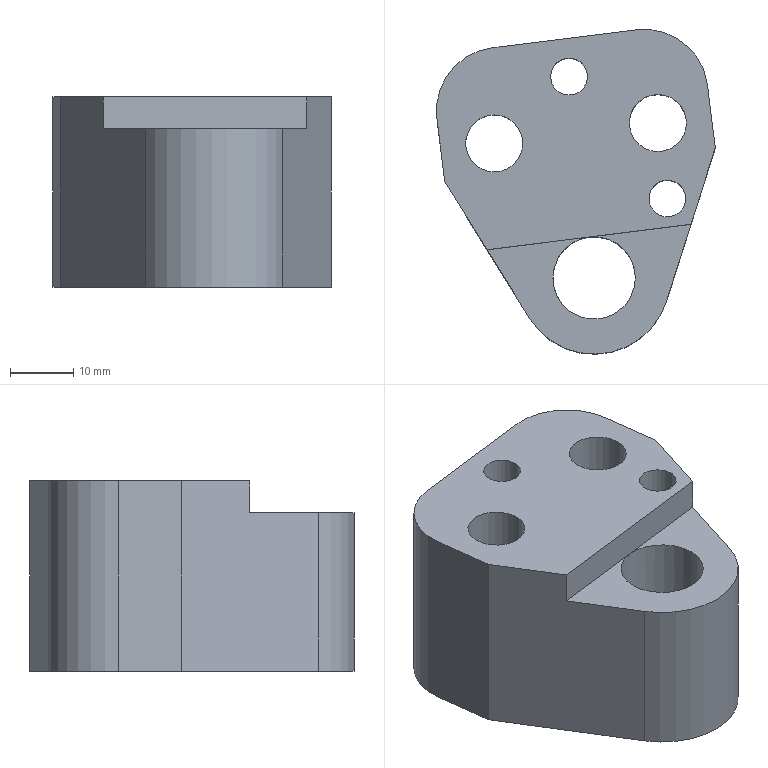Part | NX | features CP-FP 13 2 | 1 solid | 21 faces | box 43.983 x 51.207 x 30 mm | volume 37532 mm3 | plane 11 | cylinder 10 | commonest cylinder face diameters 5.8 x2 9 x2 14 x2 20 x2 13 x1 24 x1
STEP:
#1=CARTESIAN_POINT('',(623.685,-6.896,49.));
#2=VERTEX_POINT('',#1);
#3=CARTESIAN_POINT('',(624.921,-16.819,49.));
#4=VERTEX_POINT('',#3);
#5=CARTESIAN_POINT('',(622.449,3.027,49.));
#6=DIRECTION('',(0.1236,-0.9923,0.));
#7=VECTOR('',#6,1000.);
#8=LINE('',#5,#7);
#9=EDGE_CURVE('',#2,#4,#8,.T.);
#10=ORIENTED_EDGE('',*,*,#9,.F.);
#11=CARTESIAN_POINT('',(623.685,-6.896,79.));
#12=VERTEX_POINT('',#11);
#13=CARTESIAN_POINT('',(623.685,-6.896,49.));
#14=DIRECTION('',(0.,0.,1.));
#15=VECTOR('',#14,1000.);
#16=LINE('',#13,#15);
#17=EDGE_CURVE('',#2,#12,#16,.T.);
#18=ORIENTED_EDGE('',*,*,#17,.T.);
#19=CARTESIAN_POINT('',(624.921,-16.819,79.));
#20=VERTEX_POINT('',#19);
#21=CARTESIAN_POINT('',(622.449,3.027,79.));
#22=DIRECTION('',(0.1236,-0.9923,0.));
#23=VECTOR('',#22,1000.);
#24=LINE('',#21,#23);
#25=EDGE_CURVE('',#12,#20,#24,.T.);
#26=ORIENTED_EDGE('',*,*,#25,.T.);
#27=CARTESIAN_POINT('',(624.921,-16.819,49.));
#28=DIRECTION('',(0.,0.,1.));
#29=VECTOR('',#28,1000.);
#30=LINE('',#27,#29);
#31=EDGE_CURVE('',#4,#20,#30,.T.);
#32=ORIENTED_EDGE('',*,*,#31,.F.);
#33=EDGE_LOOP('',(#10,#18,#26,#32));
#34=FACE_BOUND('',#33,.T.);
#35=CARTESIAN_POINT('',(622.449,3.027,49.));
#36=DIRECTION('',(-0.9923,-0.1236,0.));
#37=DIRECTION('',(0.1236,-0.9923,0.));
#38=AXIS2_PLACEMENT_3D('',#35,#36,#37);
#39=PLANE('',#38);
#40=ADVANCED_FACE('',(#34),#39,.F.);
#41=CARTESIAN_POINT('',(621.088,-28.886,79.));
#42=VERTEX_POINT('',#41);
#43=CARTESIAN_POINT('',(621.088,-28.886,74.));
#44=VERTEX_POINT('',#43);
#45=CARTESIAN_POINT('',(621.088,-28.886,49.));
#46=DIRECTION('',(0.,0.,-1.));
#47=VECTOR('',#46,1000.);
#48=LINE('',#45,#47);
#49=EDGE_CURVE('',#42,#44,#48,.T.);
#50=ORIENTED_EDGE('',*,*,#49,.T.);
#51=CARTESIAN_POINT('',(617.248,-40.972,74.));
#52=VERTEX_POINT('',#51);
#53=CARTESIAN_POINT('',(624.921,-16.819,74.));
#54=DIRECTION('',(-0.3028,-0.9531,0.));
#55=VECTOR('',#54,1000.);
#56=LINE('',#53,#55);
#57=EDGE_CURVE('',#44,#52,#56,.T.);
#58=ORIENTED_EDGE('',*,*,#57,.T.);
#59=CARTESIAN_POINT('',(617.248,-40.972,49.));
#60=VERTEX_POINT('',#59);
#61=CARTESIAN_POINT('',(617.248,-40.972,49.));
#62=DIRECTION('',(0.,0.,1.));
#63=VECTOR('',#62,1000.);
#64=LINE('',#61,#63);
#65=EDGE_CURVE('',#60,#52,#64,.T.);
#66=ORIENTED_EDGE('',*,*,#65,.F.);
#67=CARTESIAN_POINT('',(624.921,-16.819,49.));
#68=DIRECTION('',(-0.3028,-0.9531,0.));
#69=VECTOR('',#68,1000.);
#70=LINE('',#67,#69);
#71=EDGE_CURVE('',#4,#60,#70,.T.);
#72=ORIENTED_EDGE('',*,*,#71,.F.);
#73=ORIENTED_EDGE('',*,*,#31,.T.);
#74=CARTESIAN_POINT('',(624.921,-16.819,79.));
#75=DIRECTION('',(-0.3028,-0.9531,0.));
#76=VECTOR('',#75,1000.);
#77=LINE('',#74,#76);
#78=EDGE_CURVE('',#20,#42,#77,.T.);
#79=ORIENTED_EDGE('',*,*,#78,.T.);
#80=EDGE_LOOP('',(#50,#58,#66,#72,#73,#79));
#81=FACE_BOUND('',#80,.T.);
#82=CARTESIAN_POINT('',(624.921,-16.819,49.));
#83=DIRECTION('',(-0.9531,0.3028,0.));
#84=DIRECTION('',(-0.3028,-0.9531,0.));
#85=AXIS2_PLACEMENT_3D('',#82,#83,#84);
#86=PLANE('',#85);
#87=ADVANCED_FACE('',(#81),#86,.F.);
#88=CARTESIAN_POINT('',(595.616,-43.668,74.));
#89=VERTEX_POINT('',#88);
#90=CARTESIAN_POINT('',(605.812,-37.339,74.));
#91=DIRECTION('',(0.,0.,-1.));
#92=DIRECTION('',(0.,1.,0.));
#93=AXIS2_PLACEMENT_3D('',#90,#91,#92);
#94=CIRCLE('',#93,12.);
#95=EDGE_CURVE('',#89,#52,#94,.F.);
#96=ORIENTED_EDGE('',*,*,#95,.F.);
#97=CARTESIAN_POINT('',(595.616,-43.668,49.));
#98=VERTEX_POINT('',#97);
#99=CARTESIAN_POINT('',(595.616,-43.668,49.));
#100=DIRECTION('',(0.,0.,1.));
#101=VECTOR('',#100,1000.);
#102=LINE('',#99,#101);
#103=EDGE_CURVE('',#98,#89,#102,.T.);
#104=ORIENTED_EDGE('',*,*,#103,.F.);
#105=CARTESIAN_POINT('',(605.812,-37.339,49.));
#106=DIRECTION('',(0.,0.,1.));
#107=DIRECTION('',(0.,-1.,0.));
#108=AXIS2_PLACEMENT_3D('',#105,#106,#107);
#109=CIRCLE('',#108,12.);
#110=EDGE_CURVE('',#98,#60,#109,.T.);
#111=ORIENTED_EDGE('',*,*,#110,.T.);
#112=ORIENTED_EDGE('',*,*,#65,.T.);
#113=EDGE_LOOP('',(#96,#104,#111,#112));
#114=FACE_BOUND('',#113,.T.);
#115=CARTESIAN_POINT('',(605.812,-37.339,49.));
#116=DIRECTION('',(0.,0.,1.));
#117=DIRECTION('',(0.,-1.,0.));
#118=AXIS2_PLACEMENT_3D('',#115,#116,#117);
#119=CYLINDRICAL_SURFACE('',#118,12.);
#120=ADVANCED_FACE('',(#114),#119,.T.);
#121=CARTESIAN_POINT('',(588.928,-32.893,74.));
#122=VERTEX_POINT('',#121);
#123=CARTESIAN_POINT('',(582.251,-22.136,74.));
#124=DIRECTION('',(0.5274,-0.8496,0.));
#125=VECTOR('',#124,1000.);
#126=LINE('',#123,#125);
#127=EDGE_CURVE('',#122,#89,#126,.T.);
#128=ORIENTED_EDGE('',*,*,#127,.F.);
#129=CARTESIAN_POINT('',(588.928,-32.893,79.));
#130=VERTEX_POINT('',#129);
#131=CARTESIAN_POINT('',(588.928,-32.893,49.));
#132=DIRECTION('',(0.,0.,-1.));
#133=VECTOR('',#132,1000.);
#134=LINE('',#131,#133);
#135=EDGE_CURVE('',#130,#122,#134,.T.);
#136=ORIENTED_EDGE('',*,*,#135,.F.);
#137=CARTESIAN_POINT('',(582.251,-22.136,79.));
#138=VERTEX_POINT('',#137);
#139=CARTESIAN_POINT('',(582.251,-22.136,79.));
#140=DIRECTION('',(0.5274,-0.8496,0.));
#141=VECTOR('',#140,1000.);
#142=LINE('',#139,#141);
#143=EDGE_CURVE('',#138,#130,#142,.T.);
#144=ORIENTED_EDGE('',*,*,#143,.F.);
#145=CARTESIAN_POINT('',(582.251,-22.136,49.));
#146=VERTEX_POINT('',#145);
#147=CARTESIAN_POINT('',(582.251,-22.136,49.));
#148=DIRECTION('',(0.,0.,1.));
#149=VECTOR('',#148,1000.);
#150=LINE('',#147,#149);
#151=EDGE_CURVE('',#146,#138,#150,.T.);
#152=ORIENTED_EDGE('',*,*,#151,.F.);
#153=CARTESIAN_POINT('',(582.251,-22.136,49.));
#154=DIRECTION('',(0.5274,-0.8496,0.));
#155=VECTOR('',#154,1000.);
#156=LINE('',#153,#155);
#157=EDGE_CURVE('',#146,#98,#156,.T.);
#158=ORIENTED_EDGE('',*,*,#157,.T.);
#159=ORIENTED_EDGE('',*,*,#103,.T.);
#160=EDGE_LOOP('',(#128,#136,#144,#152,#158,#159));
#161=FACE_BOUND('',#160,.T.);
#162=CARTESIAN_POINT('',(582.251,-22.136,49.));
#163=DIRECTION('',(-0.8496,-0.5274,0.));
#164=DIRECTION('',(0.5274,-0.8496,0.));
#165=AXIS2_PLACEMENT_3D('',#162,#163,#164);
#166=PLANE('',#165);
#167=ADVANCED_FACE('',(#161),#166,.T.);
#168=CARTESIAN_POINT('',(581.015,-12.212,79.));
#169=VERTEX_POINT('',#168);
#170=CARTESIAN_POINT('',(579.778,-2.289,79.));
#171=DIRECTION('',(0.1236,-0.9923,0.));
#172=VECTOR('',#171,1000.);
#173=LINE('',#170,#172);
#174=EDGE_CURVE('',#169,#138,#173,.T.);
#175=ORIENTED_EDGE('',*,*,#174,.F.);
#176=CARTESIAN_POINT('',(581.015,-12.212,49.));
#177=VERTEX_POINT('',#176);
#178=CARTESIAN_POINT('',(581.015,-12.212,49.));
#179=DIRECTION('',(0.,0.,1.));
#180=VECTOR('',#179,1000.);
#181=LINE('',#178,#180);
#182=EDGE_CURVE('',#169,#177,#181,.F.);
#183=ORIENTED_EDGE('',*,*,#182,.T.);
#184=CARTESIAN_POINT('',(579.778,-2.289,49.));
#185=DIRECTION('',(0.1236,-0.9923,0.));
#186=VECTOR('',#185,1000.);
#187=LINE('',#184,#186);
#188=EDGE_CURVE('',#177,#146,#187,.T.);
#189=ORIENTED_EDGE('',*,*,#188,.T.);
#190=ORIENTED_EDGE('',*,*,#151,.T.);
#191=EDGE_LOOP('',(#175,#183,#189,#190));
#192=FACE_BOUND('',#191,.T.);
#193=CARTESIAN_POINT('',(579.778,-2.289,49.));
#194=DIRECTION('',(-0.9923,-0.1236,0.));
#195=DIRECTION('',(0.1236,-0.9923,0.));
#196=AXIS2_PLACEMENT_3D('',#193,#194,#195);
#197=PLANE('',#196);
#198=ADVANCED_FACE('',(#192),#197,.T.);
#199=CARTESIAN_POINT('',(589.702,-1.053,79.));
#200=VERTEX_POINT('',#199);
#201=CARTESIAN_POINT('',(612.525,1.791,79.));
#202=VERTEX_POINT('',#201);
#203=CARTESIAN_POINT('',(579.778,-2.289,79.));
#204=DIRECTION('',(0.9923,0.1236,0.));
#205=VECTOR('',#204,1000.);
#206=LINE('',#203,#205);
#207=EDGE_CURVE('',#200,#202,#206,.T.);
#208=ORIENTED_EDGE('',*,*,#207,.T.);
#209=CARTESIAN_POINT('',(612.525,1.791,49.));
#210=VERTEX_POINT('',#209);
#211=CARTESIAN_POINT('',(612.525,1.791,49.));
#212=DIRECTION('',(0.,0.,1.));
#213=VECTOR('',#212,1000.);
#214=LINE('',#211,#213);
#215=EDGE_CURVE('',#202,#210,#214,.F.);
#216=ORIENTED_EDGE('',*,*,#215,.T.);
#217=CARTESIAN_POINT('',(589.702,-1.053,49.));
#218=VERTEX_POINT('',#217);
#219=CARTESIAN_POINT('',(579.778,-2.289,49.));
#220=DIRECTION('',(0.9923,0.1236,0.));
#221=VECTOR('',#220,1000.);
#222=LINE('',#219,#221);
#223=EDGE_CURVE('',#218,#210,#222,.T.);
#224=ORIENTED_EDGE('',*,*,#223,.F.);
#225=CARTESIAN_POINT('',(589.702,-1.053,79.));
#226=DIRECTION('',(0.,0.,1.));
#227=VECTOR('',#226,1000.);
#228=LINE('',#225,#227);
#229=EDGE_CURVE('',#218,#200,#228,.T.);
#230=ORIENTED_EDGE('',*,*,#229,.T.);
#231=EDGE_LOOP('',(#208,#216,#224,#230));
#232=FACE_BOUND('',#231,.T.);
#233=CARTESIAN_POINT('',(579.778,-2.289,49.));
#234=DIRECTION('',(0.1236,-0.9923,0.));
#235=DIRECTION('',(0.9923,0.1236,0.));
#236=AXIS2_PLACEMENT_3D('',#233,#234,#235);
#237=PLANE('',#236);
#238=ADVANCED_FACE('',(#232),#237,.F.);
#239=CARTESIAN_POINT('',(615.868,-19.909,49.));
#240=VERTEX_POINT('',#239);
#241=CARTESIAN_POINT('',(615.868,-12.909,49.));
#242=DIRECTION('',(0.,0.,1.));
#243=DIRECTION('',(0.,-1.,0.));
#244=AXIS2_PLACEMENT_3D('',#241,#242,#243);
#245=CIRCLE('',#244,7.);
#246=EDGE_CURVE('',#240,#240,#245,.T.);
#247=ORIENTED_EDGE('',*,*,#246,.T.);
#248=EDGE_LOOP('',(#247));
#249=FACE_BOUND('',#248,.T.);
#250=CARTESIAN_POINT('',(590.068,-23.123,49.));
#251=VERTEX_POINT('',#250);
#252=CARTESIAN_POINT('',(590.068,-16.123,49.));
#253=DIRECTION('',(0.,0.,1.));
#254=DIRECTION('',(0.,-1.,0.));
#255=AXIS2_PLACEMENT_3D('',#252,#253,#254);
#256=CIRCLE('',#255,7.);
#257=EDGE_CURVE('',#251,#251,#256,.T.);
#258=ORIENTED_EDGE('',*,*,#257,.T.);
#259=EDGE_LOOP('',(#258));
#260=FACE_BOUND('',#259,.T.);
#261=CARTESIAN_POINT('',(617.352,-27.716,49.));
#262=VERTEX_POINT('',#261);
#263=CARTESIAN_POINT('',(617.352,-24.816,49.));
#264=DIRECTION('',(0.,0.,1.));
#265=DIRECTION('',(0.,-1.,0.));
#266=AXIS2_PLACEMENT_3D('',#263,#264,#265);
#267=CIRCLE('',#266,2.9);
#268=EDGE_CURVE('',#262,#262,#267,.T.);
#269=ORIENTED_EDGE('',*,*,#268,.T.);
#270=EDGE_LOOP('',(#269));
#271=FACE_BOUND('',#270,.T.);
#272=CARTESIAN_POINT('',(601.855,-8.485,49.));
#273=VERTEX_POINT('',#272);
#274=CARTESIAN_POINT('',(601.855,-5.585,49.));
#275=DIRECTION('',(0.,0.,1.));
#276=DIRECTION('',(0.,-1.,0.));
#277=AXIS2_PLACEMENT_3D('',#274,#275,#276);
#278=CIRCLE('',#277,2.9);
#279=EDGE_CURVE('',#273,#273,#278,.T.);
#280=ORIENTED_EDGE('',*,*,#279,.T.);
#281=EDGE_LOOP('',(#280));
#282=FACE_BOUND('',#281,.T.);
#283=CARTESIAN_POINT('',(605.812,-43.839,49.));
#284=VERTEX_POINT('',#283);
#285=CARTESIAN_POINT('',(605.812,-37.339,49.));
#286=DIRECTION('',(0.,0.,1.));
#287=DIRECTION('',(0.,-1.,0.));
#288=AXIS2_PLACEMENT_3D('',#285,#286,#287);
#289=CIRCLE('',#288,6.5);
#290=EDGE_CURVE('',#284,#284,#289,.T.);
#291=ORIENTED_EDGE('',*,*,#290,.T.);
#292=EDGE_LOOP('',(#291));
#293=FACE_BOUND('',#292,.T.);
#294=ORIENTED_EDGE('',*,*,#223,.T.);
#295=CARTESIAN_POINT('',(613.762,-8.132,49.));
#296=DIRECTION('',(0.,0.,1.));
#297=DIRECTION('',(0.,-1.,0.));
#298=AXIS2_PLACEMENT_3D('',#295,#296,#297);
#299=CIRCLE('',#298,10.);
#300=EDGE_CURVE('',#210,#2,#299,.F.);
#301=ORIENTED_EDGE('',*,*,#300,.T.);
#302=ORIENTED_EDGE('',*,*,#9,.T.);
#303=ORIENTED_EDGE('',*,*,#71,.T.);
#304=ORIENTED_EDGE('',*,*,#110,.F.);
#305=ORIENTED_EDGE('',*,*,#157,.F.);
#306=ORIENTED_EDGE('',*,*,#188,.F.);
#307=CARTESIAN_POINT('',(590.938,-10.976,49.));
#308=DIRECTION('',(0.,0.,1.));
#309=DIRECTION('',(0.,-1.,0.));
#310=AXIS2_PLACEMENT_3D('',#307,#308,#309);
#311=CIRCLE('',#310,10.);
#312=EDGE_CURVE('',#177,#218,#311,.F.);
#313=ORIENTED_EDGE('',*,*,#312,.T.);
#314=EDGE_LOOP('',(#294,#301,#302,#303,#304,#305,#306,#313));
#315=FACE_BOUND('',#314,.T.);
#316=CARTESIAN_POINT('',(605.812,-37.339,49.));
#317=DIRECTION('',(0.,0.,1.));
#318=DIRECTION('',(0.,-1.,0.));
#319=AXIS2_PLACEMENT_3D('',#316,#317,#318);
#320=PLANE('',#319);
#321=ADVANCED_FACE('',(#249,#260,#271,#282,#293,#315),#320,.F.);
#322=CARTESIAN_POINT('',(615.868,-17.409,79.));
#323=VERTEX_POINT('',#322);
#324=CARTESIAN_POINT('',(615.868,-12.909,79.));
#325=DIRECTION('',(0.,0.,1.));
#326=DIRECTION('',(0.,-1.,0.));
#327=AXIS2_PLACEMENT_3D('',#324,#325,#326);
#328=CIRCLE('',#327,4.5);
#329=EDGE_CURVE('',#323,#323,#328,.T.);
#330=ORIENTED_EDGE('',*,*,#329,.F.);
#331=EDGE_LOOP('',(#330));
#332=FACE_BOUND('',#331,.T.);
#333=CARTESIAN_POINT('',(590.068,-20.623,79.));
#334=VERTEX_POINT('',#333);
#335=CARTESIAN_POINT('',(590.068,-16.123,79.));
#336=DIRECTION('',(0.,0.,1.));
#337=DIRECTION('',(0.,-1.,0.));
#338=AXIS2_PLACEMENT_3D('',#335,#336,#337);
#339=CIRCLE('',#338,4.5);
#340=EDGE_CURVE('',#334,#334,#339,.T.);
#341=ORIENTED_EDGE('',*,*,#340,.F.);
#342=EDGE_LOOP('',(#341));
#343=FACE_BOUND('',#342,.T.);
#344=CARTESIAN_POINT('',(617.352,-27.716,79.));
#345=VERTEX_POINT('',#344);
#346=CARTESIAN_POINT('',(617.352,-24.816,79.));
#347=DIRECTION('',(0.,0.,1.));
#348=DIRECTION('',(0.,-1.,0.));
#349=AXIS2_PLACEMENT_3D('',#346,#347,#348);
#350=CIRCLE('',#349,2.9);
#351=EDGE_CURVE('',#345,#345,#350,.T.);
#352=ORIENTED_EDGE('',*,*,#351,.F.);
#353=EDGE_LOOP('',(#352));
#354=FACE_BOUND('',#353,.T.);
#355=CARTESIAN_POINT('',(601.855,-8.485,79.));
#356=VERTEX_POINT('',#355);
#357=CARTESIAN_POINT('',(601.855,-5.585,79.));
#358=DIRECTION('',(0.,0.,1.));
#359=DIRECTION('',(0.,-1.,0.));
#360=AXIS2_PLACEMENT_3D('',#357,#358,#359);
#361=CIRCLE('',#360,2.9);
#362=EDGE_CURVE('',#356,#356,#361,.T.);
#363=ORIENTED_EDGE('',*,*,#362,.F.);
#364=EDGE_LOOP('',(#363));
#365=FACE_BOUND('',#364,.T.);
#366=CARTESIAN_POINT('',(605.008,-30.889,79.));
#367=DIRECTION('',(-0.9923,-0.1236,0.));
#368=VECTOR('',#367,1000.);
#369=LINE('',#366,#368);
#370=EDGE_CURVE('',#42,#130,#369,.T.);
#371=ORIENTED_EDGE('',*,*,#370,.F.);
#372=ORIENTED_EDGE('',*,*,#78,.F.);
#373=ORIENTED_EDGE('',*,*,#25,.F.);
#374=CARTESIAN_POINT('',(613.762,-8.132,79.));
#375=DIRECTION('',(0.,0.,1.));
#376=DIRECTION('',(0.,-1.,0.));
#377=AXIS2_PLACEMENT_3D('',#374,#375,#376);
#378=CIRCLE('',#377,10.);
#379=EDGE_CURVE('',#12,#202,#378,.T.);
#380=ORIENTED_EDGE('',*,*,#379,.T.);
#381=ORIENTED_EDGE('',*,*,#207,.F.);
#382=CARTESIAN_POINT('',(590.938,-10.976,79.));
#383=DIRECTION('',(0.,0.,1.));
#384=DIRECTION('',(0.,-1.,0.));
#385=AXIS2_PLACEMENT_3D('',#382,#383,#384);
#386=CIRCLE('',#385,10.);
#387=EDGE_CURVE('',#200,#169,#386,.T.);
#388=ORIENTED_EDGE('',*,*,#387,.T.);
#389=ORIENTED_EDGE('',*,*,#174,.T.);
#390=ORIENTED_EDGE('',*,*,#143,.T.);
#391=EDGE_LOOP('',(#371,#372,#373,#380,#381,#388,#389,#390));
#392=FACE_BOUND('',#391,.T.);
#393=CARTESIAN_POINT('',(605.812,-37.339,79.));
#394=DIRECTION('',(0.,0.,1.));
#395=DIRECTION('',(0.,-1.,0.));
#396=AXIS2_PLACEMENT_3D('',#393,#394,#395);
#397=PLANE('',#396);
#398=ADVANCED_FACE('',(#332,#343,#354,#365,#392),#397,.T.);
#399=ORIENTED_EDGE('',*,*,#312,.F.);
#400=ORIENTED_EDGE('',*,*,#182,.F.);
#401=ORIENTED_EDGE('',*,*,#387,.F.);
#402=ORIENTED_EDGE('',*,*,#229,.F.);
#403=EDGE_LOOP('',(#399,#400,#401,#402));
#404=FACE_BOUND('',#403,.T.);
#405=CARTESIAN_POINT('',(590.938,-10.976,49.));
#406=DIRECTION('',(0.,0.,-1.));
#407=DIRECTION('',(0.,1.,0.));
#408=AXIS2_PLACEMENT_3D('',#405,#406,#407);
#409=CYLINDRICAL_SURFACE('',#408,10.);
#410=ADVANCED_FACE('',(#404),#409,.T.);
#411=ORIENTED_EDGE('',*,*,#300,.F.);
#412=ORIENTED_EDGE('',*,*,#215,.F.);
#413=ORIENTED_EDGE('',*,*,#379,.F.);
#414=ORIENTED_EDGE('',*,*,#17,.F.);
#415=EDGE_LOOP('',(#411,#412,#413,#414));
#416=FACE_BOUND('',#415,.T.);
#417=CARTESIAN_POINT('',(613.762,-8.132,49.));
#418=DIRECTION('',(0.,0.,1.));
#419=DIRECTION('',(0.,-1.,0.));
#420=AXIS2_PLACEMENT_3D('',#417,#418,#419);
#421=CYLINDRICAL_SURFACE('',#420,10.);
#422=ADVANCED_FACE('',(#416),#421,.T.);
#423=CARTESIAN_POINT('',(605.008,-30.889,74.));
#424=VERTEX_POINT('',#423);
#425=CARTESIAN_POINT('',(605.008,-30.889,74.));
#426=DIRECTION('',(-0.9923,-0.1236,0.));
#427=VECTOR('',#426,1000.);
#428=LINE('',#425,#427);
#429=EDGE_CURVE('',#44,#424,#428,.T.);
#430=ORIENTED_EDGE('',*,*,#429,.T.);
#431=CARTESIAN_POINT('',(605.812,-37.339,74.));
#432=DIRECTION('',(0.,0.,-1.));
#433=DIRECTION('',(0.,1.,0.));
#434=AXIS2_PLACEMENT_3D('',#431,#432,#433);
#435=CIRCLE('',#434,6.5);
#436=EDGE_CURVE('',#424,#424,#435,.T.);
#437=ORIENTED_EDGE('',*,*,#436,.T.);
#438=CARTESIAN_POINT('',(605.008,-30.889,74.));
#439=DIRECTION('',(-0.9923,-0.1236,0.));
#440=VECTOR('',#439,1000.);
#441=LINE('',#438,#440);
#442=EDGE_CURVE('',#424,#122,#441,.T.);
#443=ORIENTED_EDGE('',*,*,#442,.T.);
#444=ORIENTED_EDGE('',*,*,#127,.T.);
#445=ORIENTED_EDGE('',*,*,#95,.T.);
#446=ORIENTED_EDGE('',*,*,#57,.F.);
#447=EDGE_LOOP('',(#430,#437,#443,#444,#445,#446));
#448=FACE_BOUND('',#447,.T.);
#449=CARTESIAN_POINT('',(606.213,-40.564,74.));
#450=DIRECTION('',(0.,0.,-1.));
#451=DIRECTION('',(0.1236,-0.9923,0.));
#452=AXIS2_PLACEMENT_3D('',#449,#450,#451);
#453=PLANE('',#452);
#454=ADVANCED_FACE('',(#448),#453,.F.);
#455=ORIENTED_EDGE('',*,*,#370,.T.);
#456=ORIENTED_EDGE('',*,*,#135,.T.);
#457=ORIENTED_EDGE('',*,*,#442,.F.);
#458=ORIENTED_EDGE('',*,*,#429,.F.);
#459=ORIENTED_EDGE('',*,*,#49,.F.);
#460=EDGE_LOOP('',(#455,#456,#457,#458,#459));
#461=FACE_BOUND('',#460,.T.);
#462=CARTESIAN_POINT('',(605.008,-30.889,74.));
#463=DIRECTION('',(-0.1236,0.9923,0.));
#464=DIRECTION('',(0.,0.,-1.));
#465=AXIS2_PLACEMENT_3D('',#462,#463,#464);
#466=PLANE('',#465);
#467=ADVANCED_FACE('',(#461),#466,.F.);
#468=ORIENTED_EDGE('',*,*,#436,.F.);
#469=EDGE_LOOP('',(#468));
#470=FACE_BOUND('',#469,.T.);
#471=ORIENTED_EDGE('',*,*,#290,.F.);
#472=EDGE_LOOP('',(#471));
#473=FACE_BOUND('',#472,.T.);
#474=CARTESIAN_POINT('',(605.812,-37.339,80.));
#475=DIRECTION('',(0.,0.,-1.));
#476=DIRECTION('',(0.,1.,0.));
#477=AXIS2_PLACEMENT_3D('',#474,#475,#476);
#478=CYLINDRICAL_SURFACE('',#477,6.5);
#479=ADVANCED_FACE('',(#470,#473),#478,.F.);
#480=ORIENTED_EDGE('',*,*,#362,.T.);
#481=EDGE_LOOP('',(#480));
#482=FACE_BOUND('',#481,.T.);
#483=ORIENTED_EDGE('',*,*,#279,.F.);
#484=EDGE_LOOP('',(#483));
#485=FACE_BOUND('',#484,.T.);
#486=CARTESIAN_POINT('',(601.855,-5.585,80.));
#487=DIRECTION('',(0.,0.,-1.));
#488=DIRECTION('',(0.,1.,0.));
#489=AXIS2_PLACEMENT_3D('',#486,#487,#488);
#490=CYLINDRICAL_SURFACE('',#489,2.9);
#491=ADVANCED_FACE('',(#482,#485),#490,.F.);
#492=ORIENTED_EDGE('',*,*,#351,.T.);
#493=EDGE_LOOP('',(#492));
#494=FACE_BOUND('',#493,.T.);
#495=ORIENTED_EDGE('',*,*,#268,.F.);
#496=EDGE_LOOP('',(#495));
#497=FACE_BOUND('',#496,.T.);
#498=CARTESIAN_POINT('',(617.352,-24.816,80.));
#499=DIRECTION('',(0.,0.,-1.));
#500=DIRECTION('',(0.,1.,0.));
#501=AXIS2_PLACEMENT_3D('',#498,#499,#500);
#502=CYLINDRICAL_SURFACE('',#501,2.9);
#503=ADVANCED_FACE('',(#494,#497),#502,.F.);
#504=CARTESIAN_POINT('',(590.068,-20.623,59.));
#505=VERTEX_POINT('',#504);
#506=CARTESIAN_POINT('',(590.068,-16.123,59.));
#507=DIRECTION('',(0.,0.,1.));
#508=DIRECTION('',(0.,-1.,0.));
#509=AXIS2_PLACEMENT_3D('',#506,#507,#508);
#510=CIRCLE('',#509,4.5);
#511=EDGE_CURVE('',#505,#505,#510,.F.);
#512=ORIENTED_EDGE('',*,*,#511,.T.);
#513=EDGE_LOOP('',(#512));
#514=FACE_BOUND('',#513,.T.);
#515=ORIENTED_EDGE('',*,*,#340,.T.);
#516=EDGE_LOOP('',(#515));
#517=FACE_BOUND('',#516,.T.);
#518=CARTESIAN_POINT('',(590.068,-16.123,80.));
#519=DIRECTION('',(0.,0.,-1.));
#520=DIRECTION('',(0.,1.,0.));
#521=AXIS2_PLACEMENT_3D('',#518,#519,#520);
#522=CYLINDRICAL_SURFACE('',#521,4.5);
#523=ADVANCED_FACE('',(#514,#517),#522,.F.);
#524=CARTESIAN_POINT('',(615.868,-17.409,59.));
#525=VERTEX_POINT('',#524);
#526=CARTESIAN_POINT('',(615.868,-12.909,59.));
#527=DIRECTION('',(0.,0.,1.));
#528=DIRECTION('',(0.,-1.,0.));
#529=AXIS2_PLACEMENT_3D('',#526,#527,#528);
#530=CIRCLE('',#529,4.5);
#531=EDGE_CURVE('',#525,#525,#530,.F.);
#532=ORIENTED_EDGE('',*,*,#531,.T.);
#533=EDGE_LOOP('',(#532));
#534=FACE_BOUND('',#533,.T.);
#535=ORIENTED_EDGE('',*,*,#329,.T.);
#536=EDGE_LOOP('',(#535));
#537=FACE_BOUND('',#536,.T.);
#538=CARTESIAN_POINT('',(615.868,-12.909,80.));
#539=DIRECTION('',(0.,0.,-1.));
#540=DIRECTION('',(0.,1.,0.));
#541=AXIS2_PLACEMENT_3D('',#538,#539,#540);
#542=CYLINDRICAL_SURFACE('',#541,4.5);
#543=ADVANCED_FACE('',(#534,#537),#542,.F.);
#544=CARTESIAN_POINT('',(590.068,-9.123,59.));
#545=VERTEX_POINT('',#544);
#546=CARTESIAN_POINT('',(590.068,-16.123,59.));
#547=DIRECTION('',(0.,0.,-1.));
#548=DIRECTION('',(0.,1.,0.));
#549=AXIS2_PLACEMENT_3D('',#546,#547,#548);
#550=CIRCLE('',#549,7.);
#551=EDGE_CURVE('',#545,#545,#550,.T.);
#552=ORIENTED_EDGE('',*,*,#551,.F.);
#553=EDGE_LOOP('',(#552));
#554=FACE_BOUND('',#553,.T.);
#555=ORIENTED_EDGE('',*,*,#257,.F.);
#556=EDGE_LOOP('',(#555));
#557=FACE_BOUND('',#556,.T.);
#558=CARTESIAN_POINT('',(590.068,-16.123,59.));
#559=DIRECTION('',(0.,0.,-1.));
#560=DIRECTION('',(0.,1.,0.));
#561=AXIS2_PLACEMENT_3D('',#558,#559,#560);
#562=CYLINDRICAL_SURFACE('',#561,7.);
#563=ADVANCED_FACE('',(#554,#557),#562,.F.);
#564=ORIENTED_EDGE('',*,*,#551,.T.);
#565=EDGE_LOOP('',(#564));
#566=FACE_BOUND('',#565,.T.);
#567=ORIENTED_EDGE('',*,*,#511,.F.);
#568=EDGE_LOOP('',(#567));
#569=FACE_BOUND('',#568,.T.);
#570=CARTESIAN_POINT('',(590.068,-16.123,59.));
#571=DIRECTION('',(0.,0.,1.));
#572=DIRECTION('',(0.,-1.,0.));
#573=AXIS2_PLACEMENT_3D('',#570,#571,#572);
#574=PLANE('',#573);
#575=ADVANCED_FACE('',(#566,#569),#574,.F.);
#576=CARTESIAN_POINT('',(615.868,-5.909,59.));
#577=VERTEX_POINT('',#576);
#578=CARTESIAN_POINT('',(615.868,-12.909,59.));
#579=DIRECTION('',(0.,0.,-1.));
#580=DIRECTION('',(0.,1.,0.));
#581=AXIS2_PLACEMENT_3D('',#578,#579,#580);
#582=CIRCLE('',#581,7.);
#583=EDGE_CURVE('',#577,#577,#582,.T.);
#584=ORIENTED_EDGE('',*,*,#583,.F.);
#585=EDGE_LOOP('',(#584));
#586=FACE_BOUND('',#585,.T.);
#587=ORIENTED_EDGE('',*,*,#246,.F.);
#588=EDGE_LOOP('',(#587));
#589=FACE_BOUND('',#588,.T.);
#590=CARTESIAN_POINT('',(615.868,-12.909,59.));
#591=DIRECTION('',(0.,0.,-1.));
#592=DIRECTION('',(0.,1.,0.));
#593=AXIS2_PLACEMENT_3D('',#590,#591,#592);
#594=CYLINDRICAL_SURFACE('',#593,7.);
#595=ADVANCED_FACE('',(#586,#589),#594,.F.);
#596=ORIENTED_EDGE('',*,*,#583,.T.);
#597=EDGE_LOOP('',(#596));
#598=FACE_BOUND('',#597,.T.);
#599=ORIENTED_EDGE('',*,*,#531,.F.);
#600=EDGE_LOOP('',(#599));
#601=FACE_BOUND('',#600,.T.);
#602=CARTESIAN_POINT('',(615.868,-12.909,59.));
#603=DIRECTION('',(0.,0.,1.));
#604=DIRECTION('',(0.,-1.,0.));
#605=AXIS2_PLACEMENT_3D('',#602,#603,#604);
#606=PLANE('',#605);
#607=ADVANCED_FACE('',(#598,#601),#606,.F.);
#608=CLOSED_SHELL('',(#40,#87,#120,#167,#198,#238,#321,#398,#410,#422,#454,#467,#479,#491,#503,#523,#543,#563,#575,#595,#607));
#609=MANIFOLD_SOLID_BREP('',#608);
#610=(LENGTH_UNIT()NAMED_UNIT(*)SI_UNIT(.MILLI.,.METRE.));
#611=UNCERTAINTY_MEASURE_WITH_UNIT(LENGTH_MEASURE(0.00001),#610,'','');
#612=(NAMED_UNIT(*)PLANE_ANGLE_UNIT()SI_UNIT($,.RADIAN.));
#613=(NAMED_UNIT(*)SI_UNIT($,.STERADIAN.)SOLID_ANGLE_UNIT());
#614=(GEOMETRIC_REPRESENTATION_CONTEXT(3)GLOBAL_UNCERTAINTY_ASSIGNED_CONTEXT((#611))GLOBAL_UNIT_ASSIGNED_CONTEXT((#610,#612,#613))REPRESENTATION_CONTEXT('',''));
#615=ADVANCED_BREP_SHAPE_REPRESENTATION('',(#609),#614);